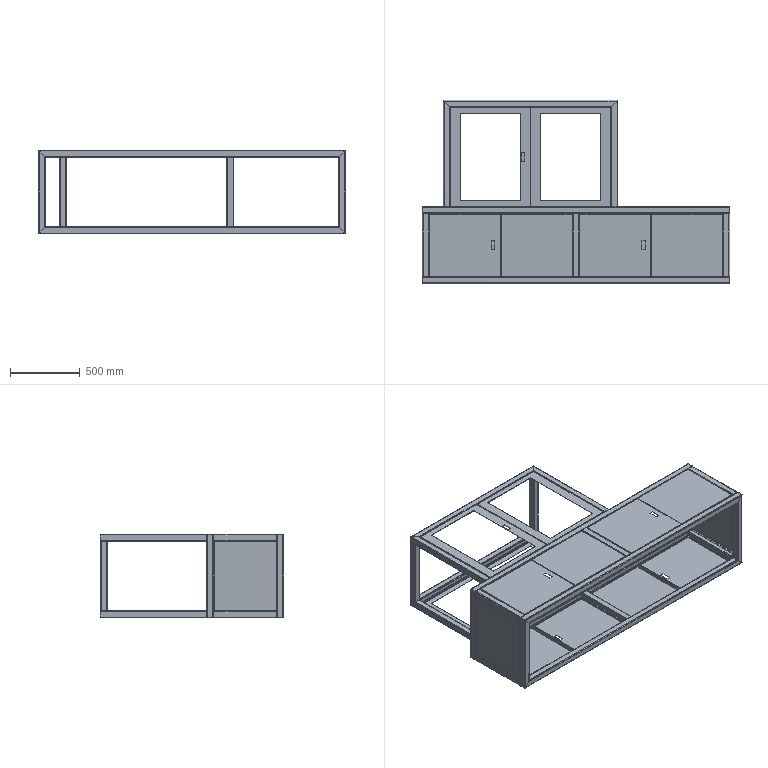Part | STEP file | 38 solids | 828 faces | box 2200 x 1312 x 600 mm | volume 17312645 mm3 | plane 540 | cylinder 288 | commonest cylinder face diameters 5.2 x96 6.4 x96 12.8 x96